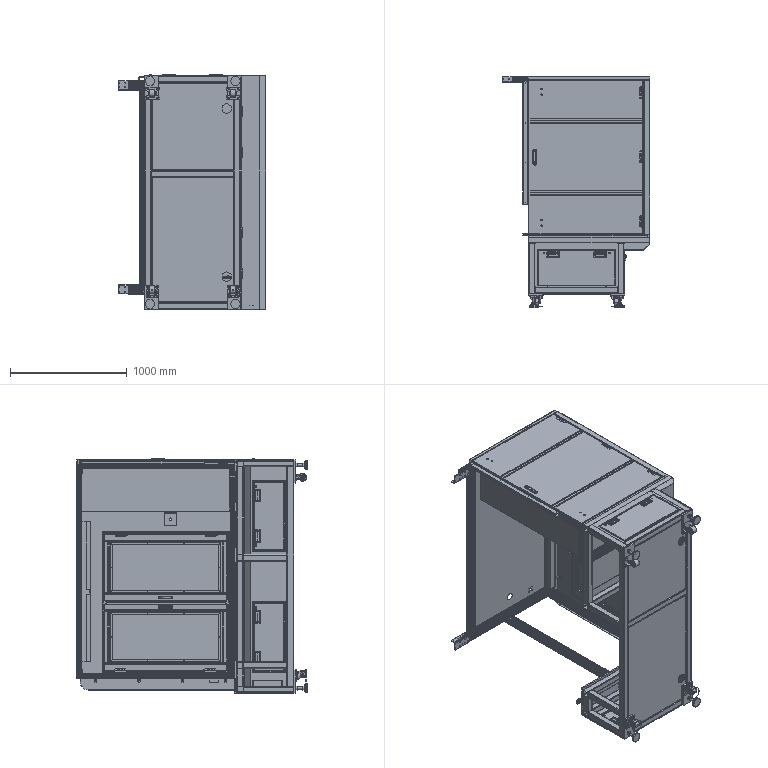Part | NX | features BREP 93 | 165 solids | 11675 faces | volume 67463582 mm3 | plane 5827 | cylinder 4900 | cone 420 | torus 284 | spline 244 | commonest cylinder face diameters 1 x764 0.4 x627 4 x460 7 x440 6 x355 5 x268